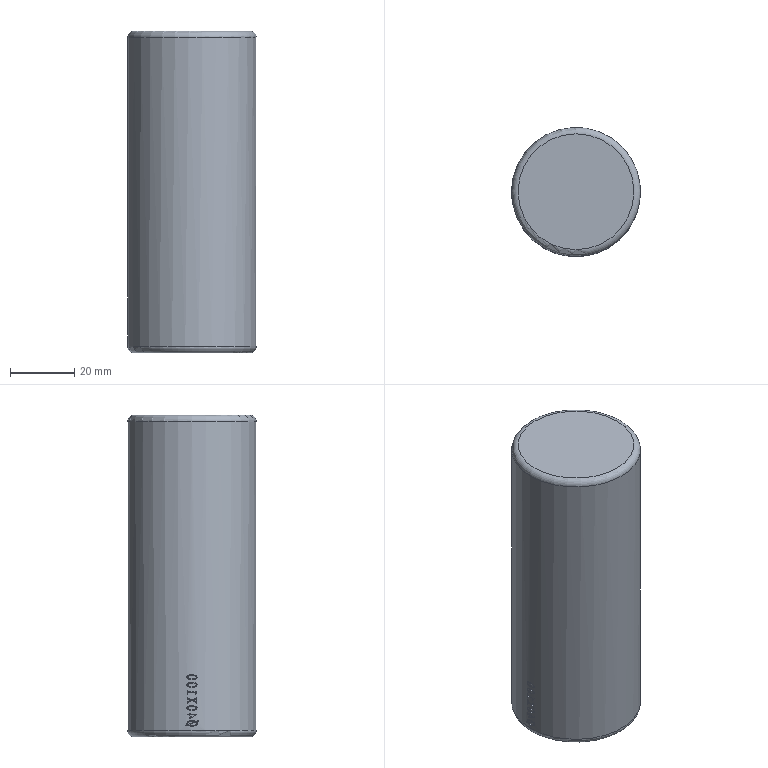Part | STEP file | solid 10 | 1 solid | 89 faces | box 40 x 40 x 100 mm | volume 109109 mm3 | plane 52 | other 26 | cylinder 8 | torus 2 | cone 1 | commonest cylinder face diameters 40 x7 20 x1